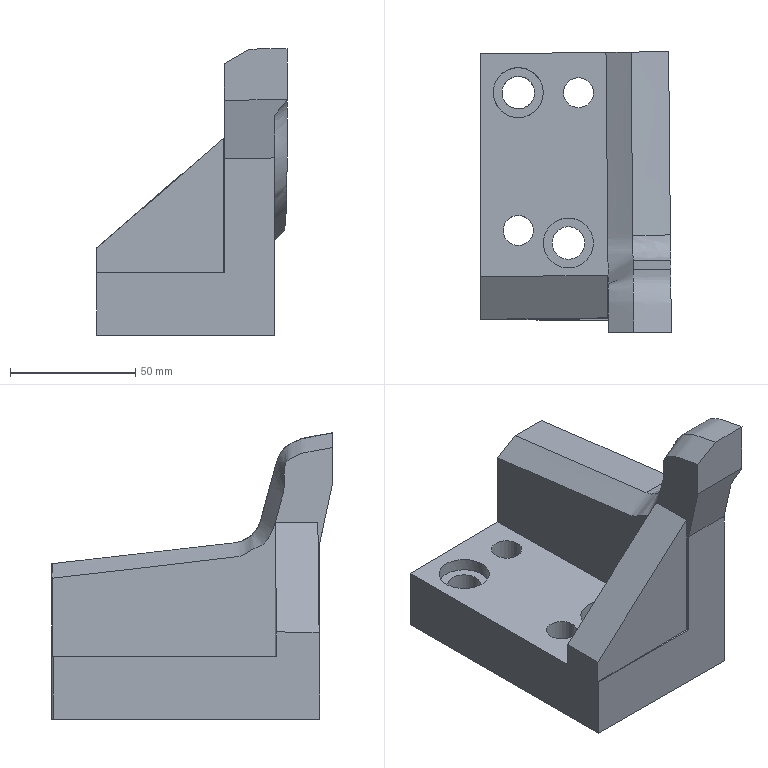Part | NX | features solid 2 | 1 solid | 30 faces | box 76.078 x 112.037 x 114.336 mm | volume 324466 mm3 | plane 14 | spline 10 | cylinder 6 | commonest cylinder face diameters 12 x2 13 x2 20 x2